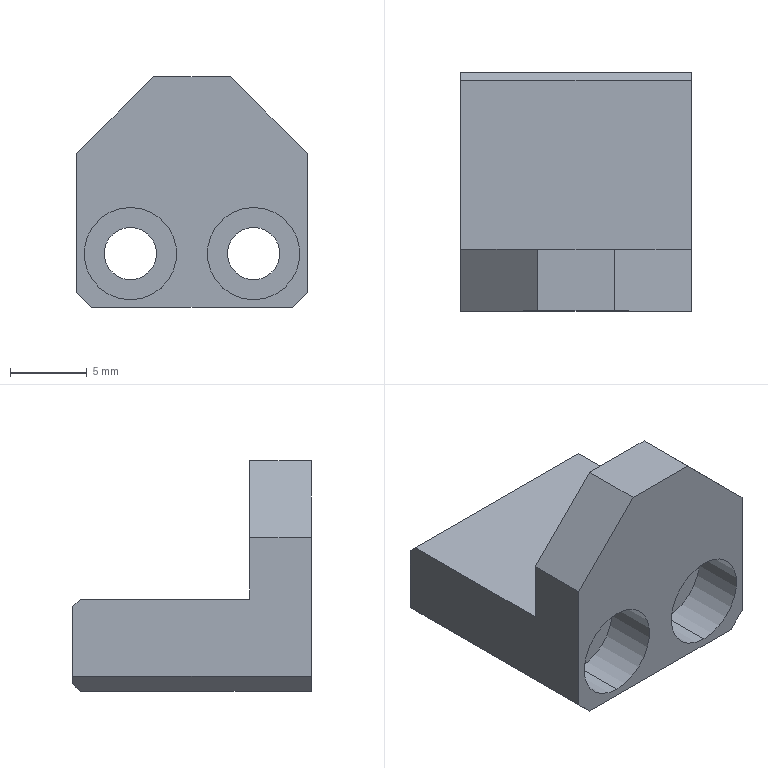Part | SolidWorks | features Chamfer 3, ICE 3, Extrusion 1, HoleWzd 1 | 1 solid | 27 faces | box 15 x 15.5 x 15 mm | volume 1371 mm3 | plane 17 | cylinder 10 | commonest cylinder face diameters 3.4 x4 6 x4 6.5 x2
STEP:
#1=CARTESIAN_POINT('',(-4.,-4.35,6.5));
#2=VERTEX_POINT('',#1);
#3=CARTESIAN_POINT('',(-4.,-4.35,0.5));
#4=VERTEX_POINT('',#3);
#5=CARTESIAN_POINT('',(-4.,-4.35,3.5));
#6=DIRECTION('',(0.,-1.,0.));
#7=DIRECTION('',(0.,0.,-1.));
#8=AXIS2_PLACEMENT_3D('',#5,#6,#7);
#9=CIRCLE('',#8,3.);
#10=EDGE_CURVE('',#2,#4,#9,.T.);
#11=ORIENTED_EDGE('',*,*,#10,.F.);
#12=CARTESIAN_POINT('',(-4.,-7.75,6.5));
#13=VERTEX_POINT('',#12);
#14=CARTESIAN_POINT('',(-4.,-7.75,6.5));
#15=DIRECTION('',(0.,-1.,0.));
#16=VECTOR('',#15,1000.);
#17=LINE('',#14,#16);
#18=EDGE_CURVE('',#2,#13,#17,.T.);
#19=ORIENTED_EDGE('',*,*,#18,.T.);
#20=CARTESIAN_POINT('',(-4.,-7.75,0.5));
#21=VERTEX_POINT('',#20);
#22=CARTESIAN_POINT('',(-4.,-7.75,3.5));
#23=DIRECTION('',(0.,-1.,0.));
#24=DIRECTION('',(0.,0.,-1.));
#25=AXIS2_PLACEMENT_3D('',#22,#23,#24);
#26=CIRCLE('',#25,3.);
#27=EDGE_CURVE('',#13,#21,#26,.T.);
#28=ORIENTED_EDGE('',*,*,#27,.T.);
#29=CARTESIAN_POINT('',(-4.,-7.75,0.5));
#30=DIRECTION('',(0.,-1.,0.));
#31=VECTOR('',#30,1000.);
#32=LINE('',#29,#31);
#33=EDGE_CURVE('',#4,#21,#32,.T.);
#34=ORIENTED_EDGE('',*,*,#33,.F.);
#35=EDGE_LOOP('',(#11,#19,#28,#34));
#36=FACE_OUTER_BOUND('',#35,.T.);
#37=CARTESIAN_POINT('',(-4.,-7.75,3.5));
#38=DIRECTION('',(0.,-1.,0.));
#39=DIRECTION('',(0.,0.,-1.));
#40=AXIS2_PLACEMENT_3D('',#37,#38,#39);
#41=CYLINDRICAL_SURFACE('',#40,3.);
#42=ADVANCED_FACE('',(#36),#41,.F.);
#43=CARTESIAN_POINT('',(-4.,7.75,5.2));
#44=VERTEX_POINT('',#43);
#45=CARTESIAN_POINT('',(-4.,7.75,1.8));
#46=VERTEX_POINT('',#45);
#47=CARTESIAN_POINT('',(-4.,7.75,3.5));
#48=DIRECTION('',(0.,-1.,0.));
#49=DIRECTION('',(0.,0.,-1.));
#50=AXIS2_PLACEMENT_3D('',#47,#48,#49);
#51=CIRCLE('',#50,1.7);
#52=EDGE_CURVE('',#44,#46,#51,.T.);
#53=ORIENTED_EDGE('',*,*,#52,.F.);
#54=CARTESIAN_POINT('',(-4.,-4.35,5.2));
#55=VERTEX_POINT('',#54);
#56=CARTESIAN_POINT('',(-4.,-7.75,5.2));
#57=DIRECTION('',(0.,-1.,0.));
#58=VECTOR('',#57,1000.);
#59=LINE('',#56,#58);
#60=EDGE_CURVE('',#44,#55,#59,.T.);
#61=ORIENTED_EDGE('',*,*,#60,.T.);
#62=CARTESIAN_POINT('',(-4.,-4.35,1.8));
#63=VERTEX_POINT('',#62);
#64=CARTESIAN_POINT('',(-4.,-4.35,3.5));
#65=DIRECTION('',(0.,-1.,0.));
#66=DIRECTION('',(0.,0.,-1.));
#67=AXIS2_PLACEMENT_3D('',#64,#65,#66);
#68=CIRCLE('',#67,1.7);
#69=EDGE_CURVE('',#55,#63,#68,.T.);
#70=ORIENTED_EDGE('',*,*,#69,.T.);
#71=CARTESIAN_POINT('',(-4.,-7.75,1.8));
#72=DIRECTION('',(0.,-1.,0.));
#73=VECTOR('',#72,1000.);
#74=LINE('',#71,#73);
#75=EDGE_CURVE('',#46,#63,#74,.T.);
#76=ORIENTED_EDGE('',*,*,#75,.F.);
#77=EDGE_LOOP('',(#53,#61,#70,#76));
#78=FACE_OUTER_BOUND('',#77,.T.);
#79=CARTESIAN_POINT('',(-4.,-7.75,3.5));
#80=DIRECTION('',(0.,-1.,0.));
#81=DIRECTION('',(0.,0.,-1.));
#82=AXIS2_PLACEMENT_3D('',#79,#80,#81);
#83=CYLINDRICAL_SURFACE('',#82,1.7);
#84=ADVANCED_FACE('',(#78),#83,.F.);
#85=CARTESIAN_POINT('',(4.,-4.35,6.5));
#86=VERTEX_POINT('',#85);
#87=CARTESIAN_POINT('',(4.,-4.35,0.5));
#88=VERTEX_POINT('',#87);
#89=CARTESIAN_POINT('',(4.,-4.35,3.5));
#90=DIRECTION('',(0.,-1.,0.));
#91=DIRECTION('',(0.,0.,-1.));
#92=AXIS2_PLACEMENT_3D('',#89,#90,#91);
#93=CIRCLE('',#92,3.);
#94=EDGE_CURVE('',#86,#88,#93,.T.);
#95=ORIENTED_EDGE('',*,*,#94,.F.);
#96=CARTESIAN_POINT('',(4.,-7.75,6.5));
#97=VERTEX_POINT('',#96);
#98=CARTESIAN_POINT('',(4.,-7.75,6.5));
#99=DIRECTION('',(0.,-1.,0.));
#100=VECTOR('',#99,1000.);
#101=LINE('',#98,#100);
#102=EDGE_CURVE('',#86,#97,#101,.T.);
#103=ORIENTED_EDGE('',*,*,#102,.T.);
#104=CARTESIAN_POINT('',(4.,-7.75,0.5));
#105=VERTEX_POINT('',#104);
#106=CARTESIAN_POINT('',(4.,-7.75,3.5));
#107=DIRECTION('',(0.,-1.,0.));
#108=DIRECTION('',(0.,0.,-1.));
#109=AXIS2_PLACEMENT_3D('',#106,#107,#108);
#110=CIRCLE('',#109,3.);
#111=EDGE_CURVE('',#97,#105,#110,.T.);
#112=ORIENTED_EDGE('',*,*,#111,.T.);
#113=CARTESIAN_POINT('',(4.,-7.75,0.5));
#114=DIRECTION('',(0.,-1.,0.));
#115=VECTOR('',#114,1000.);
#116=LINE('',#113,#115);
#117=EDGE_CURVE('',#88,#105,#116,.T.);
#118=ORIENTED_EDGE('',*,*,#117,.F.);
#119=EDGE_LOOP('',(#95,#103,#112,#118));
#120=FACE_OUTER_BOUND('',#119,.T.);
#121=CARTESIAN_POINT('',(4.,-7.75,3.5));
#122=DIRECTION('',(0.,-1.,0.));
#123=DIRECTION('',(0.,0.,-1.));
#124=AXIS2_PLACEMENT_3D('',#121,#122,#123);
#125=CYLINDRICAL_SURFACE('',#124,3.);
#126=ADVANCED_FACE('',(#120),#125,.F.);
#127=CARTESIAN_POINT('',(4.,7.75,5.2));
#128=VERTEX_POINT('',#127);
#129=CARTESIAN_POINT('',(4.,7.75,1.8));
#130=VERTEX_POINT('',#129);
#131=CARTESIAN_POINT('',(4.,7.75,3.5));
#132=DIRECTION('',(0.,-1.,0.));
#133=DIRECTION('',(0.,0.,-1.));
#134=AXIS2_PLACEMENT_3D('',#131,#132,#133);
#135=CIRCLE('',#134,1.7);
#136=EDGE_CURVE('',#128,#130,#135,.T.);
#137=ORIENTED_EDGE('',*,*,#136,.F.);
#138=CARTESIAN_POINT('',(4.,-4.35,5.2));
#139=VERTEX_POINT('',#138);
#140=CARTESIAN_POINT('',(4.,-7.75,5.2));
#141=DIRECTION('',(0.,-1.,0.));
#142=VECTOR('',#141,1000.);
#143=LINE('',#140,#142);
#144=EDGE_CURVE('',#128,#139,#143,.T.);
#145=ORIENTED_EDGE('',*,*,#144,.T.);
#146=CARTESIAN_POINT('',(4.,-4.35,1.8));
#147=VERTEX_POINT('',#146);
#148=CARTESIAN_POINT('',(4.,-4.35,3.5));
#149=DIRECTION('',(0.,-1.,0.));
#150=DIRECTION('',(0.,0.,-1.));
#151=AXIS2_PLACEMENT_3D('',#148,#149,#150);
#152=CIRCLE('',#151,1.7);
#153=EDGE_CURVE('',#139,#147,#152,.T.);
#154=ORIENTED_EDGE('',*,*,#153,.T.);
#155=CARTESIAN_POINT('',(4.,-7.75,1.8));
#156=DIRECTION('',(0.,-1.,0.));
#157=VECTOR('',#156,1000.);
#158=LINE('',#155,#157);
#159=EDGE_CURVE('',#130,#147,#158,.T.);
#160=ORIENTED_EDGE('',*,*,#159,.F.);
#161=EDGE_LOOP('',(#137,#145,#154,#160));
#162=FACE_OUTER_BOUND('',#161,.T.);
#163=CARTESIAN_POINT('',(4.,-7.75,3.5));
#164=DIRECTION('',(0.,-1.,0.));
#165=DIRECTION('',(0.,0.,-1.));
#166=AXIS2_PLACEMENT_3D('',#163,#164,#165);
#167=CYLINDRICAL_SURFACE('',#166,1.7);
#168=ADVANCED_FACE('',(#162),#167,.F.);
#169=CARTESIAN_POINT('',(0.,-4.75,7.75));
#170=VERTEX_POINT('',#169);
#171=CARTESIAN_POINT('',(0.,-4.75,14.25));
#172=VERTEX_POINT('',#171);
#173=CARTESIAN_POINT('',(0.,-4.75,11.));
#174=DIRECTION('',(0.,1.,0.));
#175=DIRECTION('',(0.,0.,1.));
#176=AXIS2_PLACEMENT_3D('',#173,#174,#175);
#177=CIRCLE('',#176,3.25);
#178=EDGE_CURVE('',#170,#172,#177,.T.);
#179=ORIENTED_EDGE('',*,*,#178,.F.);
#180=CARTESIAN_POINT('',(0.,-3.75,7.75));
#181=VERTEX_POINT('',#180);
#182=CARTESIAN_POINT('',(0.,-4.75,7.75));
#183=DIRECTION('',(0.,1.,0.));
#184=VECTOR('',#183,1000.);
#185=LINE('',#182,#184);
#186=EDGE_CURVE('',#170,#181,#185,.T.);
#187=ORIENTED_EDGE('',*,*,#186,.T.);
#188=CARTESIAN_POINT('',(0.,-3.75,14.25));
#189=VERTEX_POINT('',#188);
#190=CARTESIAN_POINT('',(0.,-3.75,11.));
#191=DIRECTION('',(0.,1.,0.));
#192=DIRECTION('',(0.,0.,1.));
#193=AXIS2_PLACEMENT_3D('',#190,#191,#192);
#194=CIRCLE('',#193,3.25);
#195=EDGE_CURVE('',#181,#189,#194,.T.);
#196=ORIENTED_EDGE('',*,*,#195,.T.);
#197=CARTESIAN_POINT('',(0.,-4.75,14.25));
#198=DIRECTION('',(0.,1.,0.));
#199=VECTOR('',#198,1000.);
#200=LINE('',#197,#199);
#201=EDGE_CURVE('',#172,#189,#200,.T.);
#202=ORIENTED_EDGE('',*,*,#201,.F.);
#203=EDGE_LOOP('',(#179,#187,#196,#202));
#204=FACE_OUTER_BOUND('',#203,.T.);
#205=CARTESIAN_POINT('',(0.,-4.75,11.));
#206=DIRECTION('',(0.,1.,0.));
#207=DIRECTION('',(0.,0.,1.));
#208=AXIS2_PLACEMENT_3D('',#205,#206,#207);
#209=CYLINDRICAL_SURFACE('',#208,3.25);
#210=ADVANCED_FACE('',(#204),#209,.F.);
#211=CARTESIAN_POINT('',(7.5,-3.75,6.));
#212=VERTEX_POINT('',#211);
#213=CARTESIAN_POINT('',(7.5,7.25,6.));
#214=VERTEX_POINT('',#213);
#215=CARTESIAN_POINT('',(7.5,-7.75,6.));
#216=DIRECTION('',(0.,1.,0.));
#217=VECTOR('',#216,1000.);
#218=LINE('',#215,#217);
#219=EDGE_CURVE('',#212,#214,#218,.T.);
#220=ORIENTED_EDGE('',*,*,#219,.T.);
#221=CARTESIAN_POINT('',(-7.5,7.25,6.));
#222=VERTEX_POINT('',#221);
#223=CARTESIAN_POINT('',(0.,7.25,6.));
#224=DIRECTION('',(-1.,0.,0.));
#225=VECTOR('',#224,1000.);
#226=LINE('',#223,#225);
#227=EDGE_CURVE('',#214,#222,#226,.T.);
#228=ORIENTED_EDGE('',*,*,#227,.T.);
#229=CARTESIAN_POINT('',(-7.5,-3.75,6.));
#230=VERTEX_POINT('',#229);
#231=CARTESIAN_POINT('',(-7.5,-7.75,6.));
#232=DIRECTION('',(0.,-1.,0.));
#233=VECTOR('',#232,1000.);
#234=LINE('',#231,#233);
#235=EDGE_CURVE('',#222,#230,#234,.T.);
#236=ORIENTED_EDGE('',*,*,#235,.T.);
#237=CARTESIAN_POINT('',(-7.5,-3.75,6.));
#238=DIRECTION('',(-1.,0.,0.));
#239=VECTOR('',#238,1000.);
#240=LINE('',#237,#239);
#241=EDGE_CURVE('',#212,#230,#240,.T.);
#242=ORIENTED_EDGE('',*,*,#241,.F.);
#243=EDGE_LOOP('',(#220,#228,#236,#242));
#244=FACE_OUTER_BOUND('',#243,.T.);
#245=CARTESIAN_POINT('',(0.,0.,6.));
#246=DIRECTION('',(0.,0.,-1.));
#247=DIRECTION('',(-1.,0.,0.));
#248=AXIS2_PLACEMENT_3D('',#245,#246,#247);
#249=PLANE('',#248);
#250=ADVANCED_FACE('',(#244),#249,.F.);
#251=CARTESIAN_POINT('',(7.5,7.75,5.5));
#252=VERTEX_POINT('',#251);
#253=CARTESIAN_POINT('',(7.5,7.75,1.));
#254=VERTEX_POINT('',#253);
#255=CARTESIAN_POINT('',(7.5,7.75,6.));
#256=DIRECTION('',(0.,0.,-1.));
#257=VECTOR('',#256,1000.);
#258=LINE('',#255,#257);
#259=EDGE_CURVE('',#252,#254,#258,.T.);
#260=ORIENTED_EDGE('',*,*,#259,.F.);
#261=CARTESIAN_POINT('',(7.5,7.25,6.));
#262=DIRECTION('',(0.,-0.7071,0.7071));
#263=VECTOR('',#262,1000.);
#264=LINE('',#261,#263);
#265=EDGE_CURVE('',#252,#214,#264,.T.);
#266=ORIENTED_EDGE('',*,*,#265,.T.);
#267=ORIENTED_EDGE('',*,*,#219,.F.);
#268=CARTESIAN_POINT('',(7.5,-3.75,10.));
#269=VERTEX_POINT('',#268);
#270=CARTESIAN_POINT('',(7.5,-3.75,15.));
#271=DIRECTION('',(0.,0.,-1.));
#272=VECTOR('',#271,1000.);
#273=LINE('',#270,#272);
#274=EDGE_CURVE('',#269,#212,#273,.T.);
#275=ORIENTED_EDGE('',*,*,#274,.F.);
#276=CARTESIAN_POINT('',(7.5,-7.75,10.));
#277=VERTEX_POINT('',#276);
#278=CARTESIAN_POINT('',(7.5,-7.75,10.));
#279=DIRECTION('',(0.,-1.,0.));
#280=VECTOR('',#279,1000.);
#281=LINE('',#278,#280);
#282=EDGE_CURVE('',#269,#277,#281,.T.);
#283=ORIENTED_EDGE('',*,*,#282,.T.);
#284=CARTESIAN_POINT('',(7.5,-7.75,1.));
#285=VERTEX_POINT('',#284);
#286=CARTESIAN_POINT('',(7.5,-7.75,6.));
#287=DIRECTION('',(0.,0.,-1.));
#288=VECTOR('',#287,1000.);
#289=LINE('',#286,#288);
#290=EDGE_CURVE('',#277,#285,#289,.T.);
#291=ORIENTED_EDGE('',*,*,#290,.T.);
#292=CARTESIAN_POINT('',(7.5,7.75,1.));
#293=DIRECTION('',(0.,1.,0.));
#294=VECTOR('',#293,1000.);
#295=LINE('',#292,#294);
#296=EDGE_CURVE('',#285,#254,#295,.T.);
#297=ORIENTED_EDGE('',*,*,#296,.T.);
#298=EDGE_LOOP('',(#260,#266,#267,#275,#283,#291,#297));
#299=FACE_OUTER_BOUND('',#298,.T.);
#300=CARTESIAN_POINT('',(7.5,-7.75,6.));
#301=DIRECTION('',(-1.,0.,0.));
#302=DIRECTION('',(0.,0.,1.));
#303=AXIS2_PLACEMENT_3D('',#300,#301,#302);
#304=PLANE('',#303);
#305=ADVANCED_FACE('',(#299),#304,.F.);
#306=CARTESIAN_POINT('',(-4.,7.75,3.5));
#307=DIRECTION('',(0.,-1.,0.));
#308=DIRECTION('',(0.,0.,-1.));
#309=AXIS2_PLACEMENT_3D('',#306,#307,#308);
#310=CIRCLE('',#309,1.7);
#311=EDGE_CURVE('',#46,#44,#310,.T.);
#312=ORIENTED_EDGE('',*,*,#311,.T.);
#313=ORIENTED_EDGE('',*,*,#52,.T.);
#314=EDGE_LOOP('',(#312,#313));
#315=FACE_BOUND('',#314,.T.);
#316=CARTESIAN_POINT('',(4.,7.75,3.5));
#317=DIRECTION('',(0.,-1.,0.));
#318=DIRECTION('',(0.,0.,-1.));
#319=AXIS2_PLACEMENT_3D('',#316,#317,#318);
#320=CIRCLE('',#319,1.7);
#321=EDGE_CURVE('',#130,#128,#320,.T.);
#322=ORIENTED_EDGE('',*,*,#321,.T.);
#323=ORIENTED_EDGE('',*,*,#136,.T.);
#324=EDGE_LOOP('',(#322,#323));
#325=FACE_BOUND('',#324,.T.);
#326=CARTESIAN_POINT('',(-7.5,7.75,5.5));
#327=VERTEX_POINT('',#326);
#328=CARTESIAN_POINT('',(-7.5,7.75,1.));
#329=VERTEX_POINT('',#328);
#330=CARTESIAN_POINT('',(-7.5,7.75,6.));
#331=DIRECTION('',(0.,0.,-1.));
#332=VECTOR('',#331,1000.);
#333=LINE('',#330,#332);
#334=EDGE_CURVE('',#327,#329,#333,.T.);
#335=ORIENTED_EDGE('',*,*,#334,.F.);
#336=CARTESIAN_POINT('',(-7.5,7.75,5.5));
#337=DIRECTION('',(1.,0.,0.));
#338=VECTOR('',#337,1000.);
#339=LINE('',#336,#338);
#340=EDGE_CURVE('',#327,#252,#339,.T.);
#341=ORIENTED_EDGE('',*,*,#340,.T.);
#342=ORIENTED_EDGE('',*,*,#259,.T.);
#343=CARTESIAN_POINT('',(7.,7.75,0.5));
#344=VERTEX_POINT('',#343);
#345=CARTESIAN_POINT('',(7.5,7.75,1.));
#346=DIRECTION('',(-0.7071,0.,-0.7071));
#347=VECTOR('',#346,1000.);
#348=LINE('',#345,#347);
#349=EDGE_CURVE('',#254,#344,#348,.T.);
#350=ORIENTED_EDGE('',*,*,#349,.T.);
#351=CARTESIAN_POINT('',(-7.,7.75,0.5));
#352=VERTEX_POINT('',#351);
#353=CARTESIAN_POINT('',(-6.5,7.75,0.5));
#354=DIRECTION('',(-1.,0.,0.));
#355=VECTOR('',#354,1000.);
#356=LINE('',#353,#355);
#357=EDGE_CURVE('',#344,#352,#356,.T.);
#358=ORIENTED_EDGE('',*,*,#357,.T.);
#359=CARTESIAN_POINT('',(-7.5,7.75,1.));
#360=DIRECTION('',(-0.7071,0.,0.7071));
#361=VECTOR('',#360,1000.);
#362=LINE('',#359,#361);
#363=EDGE_CURVE('',#352,#329,#362,.T.);
#364=ORIENTED_EDGE('',*,*,#363,.T.);
#365=EDGE_LOOP('',(#335,#341,#342,#350,#358,#364));
#366=FACE_OUTER_BOUND('',#365,.T.);
#367=CARTESIAN_POINT('',(-7.5,7.75,6.));
#368=DIRECTION('',(0.,-1.,0.));
#369=DIRECTION('',(0.,0.,-1.));
#370=AXIS2_PLACEMENT_3D('',#367,#368,#369);
#371=PLANE('',#370);
#372=ADVANCED_FACE('',(#315,#325,#366),#371,.F.);
#373=ORIENTED_EDGE('',*,*,#235,.F.);
#374=CARTESIAN_POINT('',(-7.5,7.25,6.));
#375=DIRECTION('',(0.,0.7071,-0.7071));
#376=VECTOR('',#375,1000.);
#377=LINE('',#374,#376);
#378=EDGE_CURVE('',#222,#327,#377,.T.);
#379=ORIENTED_EDGE('',*,*,#378,.T.);
#380=ORIENTED_EDGE('',*,*,#334,.T.);
#381=CARTESIAN_POINT('',(-7.5,-7.75,1.));
#382=VERTEX_POINT('',#381);
#383=CARTESIAN_POINT('',(-7.5,-7.75,1.));
#384=DIRECTION('',(0.,-1.,0.));
#385=VECTOR('',#384,1000.);
#386=LINE('',#383,#385);
#387=EDGE_CURVE('',#329,#382,#386,.T.);
#388=ORIENTED_EDGE('',*,*,#387,.T.);
#389=CARTESIAN_POINT('',(-7.5,-7.75,10.));
#390=VERTEX_POINT('',#389);
#391=CARTESIAN_POINT('',(-7.5,-7.75,6.));
#392=DIRECTION('',(0.,0.,-1.));
#393=VECTOR('',#392,1000.);
#394=LINE('',#391,#393);
#395=EDGE_CURVE('',#390,#382,#394,.T.);
#396=ORIENTED_EDGE('',*,*,#395,.F.);
#397=CARTESIAN_POINT('',(-7.5,-3.75,10.));
#398=VERTEX_POINT('',#397);
#399=CARTESIAN_POINT('',(-7.5,-7.75,10.));
#400=DIRECTION('',(0.,1.,0.));
#401=VECTOR('',#400,1000.);
#402=LINE('',#399,#401);
#403=EDGE_CURVE('',#390,#398,#402,.T.);
#404=ORIENTED_EDGE('',*,*,#403,.T.);
#405=CARTESIAN_POINT('',(-7.5,-3.75,15.));
#406=DIRECTION('',(0.,0.,-1.));
#407=VECTOR('',#406,1000.);
#408=LINE('',#405,#407);
#409=EDGE_CURVE('',#398,#230,#408,.T.);
#410=ORIENTED_EDGE('',*,*,#409,.T.);
#411=EDGE_LOOP('',(#373,#379,#380,#388,#396,#404,#410));
#412=FACE_OUTER_BOUND('',#411,.T.);
#413=CARTESIAN_POINT('',(-7.5,-7.75,6.));
#414=DIRECTION('',(1.,0.,0.));
#415=DIRECTION('',(0.,0.,-1.));
#416=AXIS2_PLACEMENT_3D('',#413,#414,#415);
#417=PLANE('',#416);
#418=ADVANCED_FACE('',(#412),#417,.F.);
#419=CARTESIAN_POINT('',(-4.,-7.75,3.5));
#420=DIRECTION('',(0.,-1.,0.));
#421=DIRECTION('',(0.,0.,-1.));
#422=AXIS2_PLACEMENT_3D('',#419,#420,#421);
#423=CIRCLE('',#422,3.);
#424=EDGE_CURVE('',#21,#13,#423,.T.);
#425=ORIENTED_EDGE('',*,*,#424,.F.);
#426=ORIENTED_EDGE('',*,*,#27,.F.);
#427=EDGE_LOOP('',(#425,#426));
#428=FACE_BOUND('',#427,.T.);
#429=CARTESIAN_POINT('',(4.,-7.75,3.5));
#430=DIRECTION('',(0.,-1.,0.));
#431=DIRECTION('',(0.,0.,-1.));
#432=AXIS2_PLACEMENT_3D('',#429,#430,#431);
#433=CIRCLE('',#432,3.);
#434=EDGE_CURVE('',#105,#97,#433,.T.);
#435=ORIENTED_EDGE('',*,*,#434,.F.);
#436=ORIENTED_EDGE('',*,*,#111,.F.);
#437=EDGE_LOOP('',(#435,#436));
#438=FACE_BOUND('',#437,.T.);
#439=CARTESIAN_POINT('',(-6.5,-7.75,0.));
#440=VERTEX_POINT('',#439);
#441=CARTESIAN_POINT('',(6.5,-7.75,0.));
#442=VERTEX_POINT('',#441);
#443=CARTESIAN_POINT('',(-7.5,-7.75,0.));
#444=DIRECTION('',(1.,0.,0.));
#445=VECTOR('',#444,1000.);
#446=LINE('',#443,#445);
#447=EDGE_CURVE('',#440,#442,#446,.T.);
#448=ORIENTED_EDGE('',*,*,#447,.T.);
#449=CARTESIAN_POINT('',(7.5,-7.75,1.));
#450=DIRECTION('',(0.7071,0.,0.7071));
#451=VECTOR('',#450,1000.);
#452=LINE('',#449,#451);
#453=EDGE_CURVE('',#442,#285,#452,.T.);
#454=ORIENTED_EDGE('',*,*,#453,.T.);
#455=ORIENTED_EDGE('',*,*,#290,.F.);
#456=CARTESIAN_POINT('',(2.5,-7.75,15.));
#457=VERTEX_POINT('',#456);
#458=CARTESIAN_POINT('',(2.5,-7.75,15.));
#459=DIRECTION('',(-0.7071,0.,0.7071));
#460=VECTOR('',#459,1000.);
#461=LINE('',#458,#460);
#462=EDGE_CURVE('',#277,#457,#461,.T.);
#463=ORIENTED_EDGE('',*,*,#462,.T.);
#464=CARTESIAN_POINT('',(-2.5,-7.75,15.));
#465=VERTEX_POINT('',#464);
#466=CARTESIAN_POINT('',(-7.5,-7.75,15.));
#467=DIRECTION('',(1.,0.,0.));
#468=VECTOR('',#467,1000.);
#469=LINE('',#466,#468);
#470=EDGE_CURVE('',#465,#457,#469,.T.);
#471=ORIENTED_EDGE('',*,*,#470,.F.);
#472=CARTESIAN_POINT('',(-2.5,-7.75,15.));
#473=DIRECTION('',(-0.7071,0.,-0.7071));
#474=VECTOR('',#473,1000.);
#475=LINE('',#472,#474);
#476=EDGE_CURVE('',#465,#390,#475,.T.);
#477=ORIENTED_EDGE('',*,*,#476,.T.);
#478=ORIENTED_EDGE('',*,*,#395,.T.);
#479=CARTESIAN_POINT('',(-7.5,-7.75,1.));
#480=DIRECTION('',(0.7071,0.,-0.7071));
#481=VECTOR('',#480,1000.);
#482=LINE('',#479,#481);
#483=EDGE_CURVE('',#382,#440,#482,.T.);
#484=ORIENTED_EDGE('',*,*,#483,.T.);
#485=EDGE_LOOP('',(#448,#454,#455,#463,#471,#477,#478,#484));
#486=FACE_OUTER_BOUND('',#485,.T.);
#487=CARTESIAN_POINT('',(-7.5,-7.75,6.));
#488=DIRECTION('',(0.,1.,0.));
#489=DIRECTION('',(0.,0.,1.));
#490=AXIS2_PLACEMENT_3D('',#487,#488,#489);
#491=PLANE('',#490);
#492=ADVANCED_FACE('',(#428,#438,#486),#491,.F.);
#493=CARTESIAN_POINT('',(-6.5,7.25,0.));
#494=VERTEX_POINT('',#493);
#495=CARTESIAN_POINT('',(-6.5,7.75,0.));
#496=DIRECTION('',(0.,1.,0.));
#497=VECTOR('',#496,1000.);
#498=LINE('',#495,#497);
#499=EDGE_CURVE('',#440,#494,#498,.T.);
#500=ORIENTED_EDGE('',*,*,#499,.T.);
#501=CARTESIAN_POINT('',(6.5,7.25,0.));
#502=VERTEX_POINT('',#501);
#503=CARTESIAN_POINT('',(6.5,7.25,0.));
#504=DIRECTION('',(1.,0.,0.));
#505=VECTOR('',#504,1000.);
#506=LINE('',#503,#505);
#507=EDGE_CURVE('',#494,#502,#506,.T.);
#508=ORIENTED_EDGE('',*,*,#507,.T.);
#509=CARTESIAN_POINT('',(6.5,-7.75,0.));
#510=DIRECTION('',(0.,-1.,0.));
#511=VECTOR('',#510,1000.);
#512=LINE('',#509,#511);
#513=EDGE_CURVE('',#502,#442,#512,.T.);
#514=ORIENTED_EDGE('',*,*,#513,.T.);
#515=ORIENTED_EDGE('',*,*,#447,.F.);
#516=EDGE_LOOP('',(#500,#508,#514,#515));
#517=FACE_OUTER_BOUND('',#516,.T.);
#518=CARTESIAN_POINT('',(0.,0.,0.));
#519=DIRECTION('',(0.,0.,-1.));
#520=DIRECTION('',(-1.,0.,0.));
#521=AXIS2_PLACEMENT_3D('',#518,#519,#520);
#522=PLANE('',#521);
#523=ADVANCED_FACE('',(#517),#522,.T.);
#524=CARTESIAN_POINT('',(0.,-3.75,11.));
#525=DIRECTION('',(0.,1.,0.));
#526=DIRECTION('',(0.,0.,1.));
#527=AXIS2_PLACEMENT_3D('',#524,#525,#526);
#528=CIRCLE('',#527,3.25);
#529=EDGE_CURVE('',#189,#181,#528,.T.);
#530=ORIENTED_EDGE('',*,*,#529,.F.);
#531=ORIENTED_EDGE('',*,*,#195,.F.);
#532=EDGE_LOOP('',(#530,#531));
#533=FACE_BOUND('',#532,.T.);
#534=ORIENTED_EDGE('',*,*,#409,.F.);
#535=CARTESIAN_POINT('',(-2.5,-3.75,15.));
#536=VERTEX_POINT('',#535);
#537=CARTESIAN_POINT('',(-2.5,-3.75,15.));
#538=DIRECTION('',(0.7071,0.,0.7071));
#539=VECTOR('',#538,1000.);
#540=LINE('',#537,#539);
#541=EDGE_CURVE('',#398,#536,#540,.T.);
#542=ORIENTED_EDGE('',*,*,#541,.T.);
#543=CARTESIAN_POINT('',(2.5,-3.75,15.));
#544=VERTEX_POINT('',#543);
#545=CARTESIAN_POINT('',(-7.5,-3.75,15.));
#546=DIRECTION('',(-1.,0.,0.));
#547=VECTOR('',#546,1000.);
#548=LINE('',#545,#547);
#549=EDGE_CURVE('',#544,#536,#548,.T.);
#550=ORIENTED_EDGE('',*,*,#549,.F.);
#551=CARTESIAN_POINT('',(2.5,-3.75,15.));
#552=DIRECTION('',(0.7071,0.,-0.7071));
#553=VECTOR('',#552,1000.);
#554=LINE('',#551,#553);
#555=EDGE_CURVE('',#544,#269,#554,.T.);
#556=ORIENTED_EDGE('',*,*,#555,.T.);
#557=ORIENTED_EDGE('',*,*,#274,.T.);
#558=ORIENTED_EDGE('',*,*,#241,.T.);
#559=EDGE_LOOP('',(#534,#542,#550,#556,#557,#558));
#560=FACE_OUTER_BOUND('',#559,.T.);
#561=CARTESIAN_POINT('',(-7.5,-3.75,15.));
#562=DIRECTION('',(0.,-1.,0.));
#563=DIRECTION('',(0.,0.,-1.));
#564=AXIS2_PLACEMENT_3D('',#561,#562,#563);
#565=PLANE('',#564);
#566=ADVANCED_FACE('',(#533,#560),#565,.F.);
#567=ORIENTED_EDGE('',*,*,#549,.T.);
#568=CARTESIAN_POINT('',(-2.5,0.,15.));
#569=DIRECTION('',(0.,-1.,0.));
#570=VECTOR('',#569,1000.);
#571=LINE('',#568,#570);
#572=EDGE_CURVE('',#536,#465,#571,.T.);
#573=ORIENTED_EDGE('',*,*,#572,.T.);
#574=ORIENTED_EDGE('',*,*,#470,.T.);
#575=CARTESIAN_POINT('',(2.5,0.,15.));
#576=DIRECTION('',(0.,1.,0.));
#577=VECTOR('',#576,1000.);
#578=LINE('',#575,#577);
#579=EDGE_CURVE('',#457,#544,#578,.T.);
#580=ORIENTED_EDGE('',*,*,#579,.T.);
#581=EDGE_LOOP('',(#567,#573,#574,#580));
#582=FACE_OUTER_BOUND('',#581,.T.);
#583=CARTESIAN_POINT('',(0.,0.,15.));
#584=DIRECTION('',(0.,0.,-1.));
#585=DIRECTION('',(-1.,0.,0.));
#586=AXIS2_PLACEMENT_3D('',#583,#584,#585);
#587=PLANE('',#586);
#588=ADVANCED_FACE('',(#582),#587,.F.);
#589=ORIENTED_EDGE('',*,*,#186,.F.);
#590=CARTESIAN_POINT('',(0.,-4.75,11.));
#591=DIRECTION('',(0.,1.,0.));
#592=DIRECTION('',(0.,0.,1.));
#593=AXIS2_PLACEMENT_3D('',#590,#591,#592);
#594=CIRCLE('',#593,3.25);
#595=EDGE_CURVE('',#172,#170,#594,.T.);
#596=ORIENTED_EDGE('',*,*,#595,.F.);
#597=ORIENTED_EDGE('',*,*,#201,.T.);
#598=ORIENTED_EDGE('',*,*,#529,.T.);
#599=EDGE_LOOP('',(#589,#596,#597,#598));
#600=FACE_OUTER_BOUND('',#599,.T.);
#601=CARTESIAN_POINT('',(0.,-4.75,11.));
#602=DIRECTION('',(0.,1.,0.));
#603=DIRECTION('',(0.,0.,1.));
#604=AXIS2_PLACEMENT_3D('',#601,#602,#603);
#605=CYLINDRICAL_SURFACE('',#604,3.25);
#606=ADVANCED_FACE('',(#600),#605,.F.);
#607=ORIENTED_EDGE('',*,*,#595,.T.);
#608=ORIENTED_EDGE('',*,*,#178,.T.);
#609=EDGE_LOOP('',(#607,#608));
#610=FACE_OUTER_BOUND('',#609,.T.);
#611=CARTESIAN_POINT('',(0.,-4.75,11.));
#612=DIRECTION('',(0.,1.,0.));
#613=DIRECTION('',(0.,0.,1.));
#614=AXIS2_PLACEMENT_3D('',#611,#612,#613);
#615=PLANE('',#614);
#616=ADVANCED_FACE('',(#610),#615,.T.);
#617=ORIENTED_EDGE('',*,*,#144,.F.);
#618=ORIENTED_EDGE('',*,*,#321,.F.);
#619=ORIENTED_EDGE('',*,*,#159,.T.);
#620=CARTESIAN_POINT('',(4.,-4.35,3.5));
#621=DIRECTION('',(0.,-1.,0.));
#622=DIRECTION('',(0.,0.,-1.));
#623=AXIS2_PLACEMENT_3D('',#620,#621,#622);
#624=CIRCLE('',#623,1.7);
#625=EDGE_CURVE('',#147,#139,#624,.T.);
#626=ORIENTED_EDGE('',*,*,#625,.T.);
#627=EDGE_LOOP('',(#617,#618,#619,#626));
#628=FACE_OUTER_BOUND('',#627,.T.);
#629=CARTESIAN_POINT('',(4.,-7.75,3.5));
#630=DIRECTION('',(0.,-1.,0.));
#631=DIRECTION('',(0.,0.,-1.));
#632=AXIS2_PLACEMENT_3D('',#629,#630,#631);
#633=CYLINDRICAL_SURFACE('',#632,1.7);
#634=ADVANCED_FACE('',(#628),#633,.F.);
#635=ORIENTED_EDGE('',*,*,#625,.F.);
#636=ORIENTED_EDGE('',*,*,#153,.F.);
#637=EDGE_LOOP('',(#635,#636));
#638=FACE_BOUND('',#637,.T.);
#639=CARTESIAN_POINT('',(4.,-4.35,3.5));
#640=DIRECTION('',(0.,-1.,0.));
#641=DIRECTION('',(0.,0.,-1.));
#642=AXIS2_PLACEMENT_3D('',#639,#640,#641);
#643=CIRCLE('',#642,3.);
#644=EDGE_CURVE('',#88,#86,#643,.T.);
#645=ORIENTED_EDGE('',*,*,#644,.T.);
#646=ORIENTED_EDGE('',*,*,#94,.T.);
#647=EDGE_LOOP('',(#645,#646));
#648=FACE_OUTER_BOUND('',#647,.T.);
#649=CARTESIAN_POINT('',(5.7,-4.35,3.5));
#650=DIRECTION('',(0.,1.,0.));
#651=DIRECTION('',(0.,0.,1.));
#652=AXIS2_PLACEMENT_3D('',#649,#650,#651);
#653=PLANE('',#652);
#654=ADVANCED_FACE('',(#638,#648),#653,.F.);
#655=ORIENTED_EDGE('',*,*,#102,.F.);
#656=ORIENTED_EDGE('',*,*,#644,.F.);
#657=ORIENTED_EDGE('',*,*,#117,.T.);
#658=ORIENTED_EDGE('',*,*,#434,.T.);
#659=EDGE_LOOP('',(#655,#656,#657,#658));
#660=FACE_OUTER_BOUND('',#659,.T.);
#661=CARTESIAN_POINT('',(4.,-7.75,3.5));
#662=DIRECTION('',(0.,-1.,0.));
#663=DIRECTION('',(0.,0.,-1.));
#664=AXIS2_PLACEMENT_3D('',#661,#662,#663);
#665=CYLINDRICAL_SURFACE('',#664,3.);
#666=ADVANCED_FACE('',(#660),#665,.F.);
#667=ORIENTED_EDGE('',*,*,#60,.F.);
#668=ORIENTED_EDGE('',*,*,#311,.F.);
#669=ORIENTED_EDGE('',*,*,#75,.T.);
#670=CARTESIAN_POINT('',(-4.,-4.35,3.5));
#671=DIRECTION('',(0.,-1.,0.));
#672=DIRECTION('',(0.,0.,-1.));
#673=AXIS2_PLACEMENT_3D('',#670,#671,#672);
#674=CIRCLE('',#673,1.7);
#675=EDGE_CURVE('',#63,#55,#674,.T.);
#676=ORIENTED_EDGE('',*,*,#675,.T.);
#677=EDGE_LOOP('',(#667,#668,#669,#676));
#678=FACE_OUTER_BOUND('',#677,.T.);
#679=CARTESIAN_POINT('',(-4.,-7.75,3.5));
#680=DIRECTION('',(0.,-1.,0.));
#681=DIRECTION('',(0.,0.,-1.));
#682=AXIS2_PLACEMENT_3D('',#679,#680,#681);
#683=CYLINDRICAL_SURFACE('',#682,1.7);
#684=ADVANCED_FACE('',(#678),#683,.F.);
#685=ORIENTED_EDGE('',*,*,#675,.F.);
#686=ORIENTED_EDGE('',*,*,#69,.F.);
#687=EDGE_LOOP('',(#685,#686));
#688=FACE_BOUND('',#687,.T.);
#689=CARTESIAN_POINT('',(-4.,-4.35,3.5));
#690=DIRECTION('',(0.,-1.,0.));
#691=DIRECTION('',(0.,0.,-1.));
#692=AXIS2_PLACEMENT_3D('',#689,#690,#691);
#693=CIRCLE('',#692,3.);
#694=EDGE_CURVE('',#4,#2,#693,.T.);
#695=ORIENTED_EDGE('',*,*,#694,.T.);
#696=ORIENTED_EDGE('',*,*,#10,.T.);
#697=EDGE_LOOP('',(#695,#696));
#698=FACE_OUTER_BOUND('',#697,.T.);
#699=CARTESIAN_POINT('',(-2.3,-4.35,3.5));
#700=DIRECTION('',(0.,1.,0.));
#701=DIRECTION('',(0.,0.,1.));
#702=AXIS2_PLACEMENT_3D('',#699,#700,#701);
#703=PLANE('',#702);
#704=ADVANCED_FACE('',(#688,#698),#703,.F.);
#705=ORIENTED_EDGE('',*,*,#18,.F.);
#706=ORIENTED_EDGE('',*,*,#694,.F.);
#707=ORIENTED_EDGE('',*,*,#33,.T.);
#708=ORIENTED_EDGE('',*,*,#424,.T.);
#709=EDGE_LOOP('',(#705,#706,#707,#708));
#710=FACE_OUTER_BOUND('',#709,.T.);
#711=CARTESIAN_POINT('',(-4.,-7.75,3.5));
#712=DIRECTION('',(0.,-1.,0.));
#713=DIRECTION('',(0.,0.,-1.));
#714=AXIS2_PLACEMENT_3D('',#711,#712,#713);
#715=CYLINDRICAL_SURFACE('',#714,3.);
#716=ADVANCED_FACE('',(#710),#715,.F.);
#717=ORIENTED_EDGE('',*,*,#541,.F.);
#718=ORIENTED_EDGE('',*,*,#403,.F.);
#719=ORIENTED_EDGE('',*,*,#476,.F.);
#720=ORIENTED_EDGE('',*,*,#572,.F.);
#721=EDGE_LOOP('',(#717,#718,#719,#720));
#722=FACE_OUTER_BOUND('',#721,.T.);
#723=CARTESIAN_POINT('',(-2.5,0.,15.));
#724=DIRECTION('',(0.7071,0.,-0.7071));
#725=DIRECTION('',(0.,-1.,0.));
#726=AXIS2_PLACEMENT_3D('',#723,#724,#725);
#727=PLANE('',#726);
#728=ADVANCED_FACE('',(#722),#727,.F.);
#729=ORIENTED_EDGE('',*,*,#462,.F.);
#730=ORIENTED_EDGE('',*,*,#282,.F.);
#731=ORIENTED_EDGE('',*,*,#555,.F.);
#732=ORIENTED_EDGE('',*,*,#579,.F.);
#733=EDGE_LOOP('',(#729,#730,#731,#732));
#734=FACE_OUTER_BOUND('',#733,.T.);
#735=CARTESIAN_POINT('',(2.5,0.,15.));
#736=DIRECTION('',(-0.7071,0.,-0.7071));
#737=DIRECTION('',(0.,1.,0.));
#738=AXIS2_PLACEMENT_3D('',#735,#736,#737);
#739=PLANE('',#738);
#740=ADVANCED_FACE('',(#734),#739,.F.);
#741=ORIENTED_EDGE('',*,*,#513,.F.);
#742=CARTESIAN_POINT('',(2.167,2.917,-4.333));
#743=DIRECTION('',(0.5774,0.5774,0.5774));
#744=VECTOR('',#743,1000.);
#745=LINE('',#742,#744);
#746=EDGE_CURVE('',#502,#344,#745,.T.);
#747=ORIENTED_EDGE('',*,*,#746,.T.);
#748=ORIENTED_EDGE('',*,*,#349,.F.);
#749=ORIENTED_EDGE('',*,*,#296,.F.);
#750=ORIENTED_EDGE('',*,*,#453,.F.);
#751=EDGE_LOOP('',(#741,#747,#748,#749,#750));
#752=FACE_OUTER_BOUND('',#751,.T.);
#753=CARTESIAN_POINT('',(7.5,-7.75,1.));
#754=DIRECTION('',(0.7071,0.,-0.7071));
#755=DIRECTION('',(0.,-1.,0.));
#756=AXIS2_PLACEMENT_3D('',#753,#754,#755);
#757=PLANE('',#756);
#758=ADVANCED_FACE('',(#752),#757,.T.);
#759=ORIENTED_EDGE('',*,*,#363,.F.);
#760=CARTESIAN_POINT('',(-2.167,2.917,-4.333));
#761=DIRECTION('',(0.5774,-0.5774,-0.5774));
#762=VECTOR('',#761,1000.);
#763=LINE('',#760,#762);
#764=EDGE_CURVE('',#352,#494,#763,.T.);
#765=ORIENTED_EDGE('',*,*,#764,.T.);
#766=ORIENTED_EDGE('',*,*,#499,.F.);
#767=ORIENTED_EDGE('',*,*,#483,.F.);
#768=ORIENTED_EDGE('',*,*,#387,.F.);
#769=EDGE_LOOP('',(#759,#765,#766,#767,#768));
#770=FACE_OUTER_BOUND('',#769,.T.);
#771=CARTESIAN_POINT('',(-7.5,-7.75,1.));
#772=DIRECTION('',(-0.7071,0.,-0.7071));
#773=DIRECTION('',(0.,1.,0.));
#774=AXIS2_PLACEMENT_3D('',#771,#772,#773);
#775=PLANE('',#774);
#776=ADVANCED_FACE('',(#770),#775,.T.);
#777=ORIENTED_EDGE('',*,*,#265,.F.);
#778=ORIENTED_EDGE('',*,*,#340,.F.);
#779=ORIENTED_EDGE('',*,*,#378,.F.);
#780=ORIENTED_EDGE('',*,*,#227,.F.);
#781=EDGE_LOOP('',(#777,#778,#779,#780));
#782=FACE_OUTER_BOUND('',#781,.T.);
#783=CARTESIAN_POINT('',(0.,7.25,6.));
#784=DIRECTION('',(0.,-0.7071,-0.7071));
#785=DIRECTION('',(-1.,0.,0.));
#786=AXIS2_PLACEMENT_3D('',#783,#784,#785);
#787=PLANE('',#786);
#788=ADVANCED_FACE('',(#782),#787,.F.);
#789=ORIENTED_EDGE('',*,*,#746,.F.);
#790=ORIENTED_EDGE('',*,*,#507,.F.);
#791=ORIENTED_EDGE('',*,*,#764,.F.);
#792=ORIENTED_EDGE('',*,*,#357,.F.);
#793=EDGE_LOOP('',(#789,#790,#791,#792));
#794=FACE_OUTER_BOUND('',#793,.T.);
#795=CARTESIAN_POINT('',(-7.5,7.75,0.5));
#796=DIRECTION('',(0.,0.7071,-0.7071));
#797=DIRECTION('',(1.,0.,0.));
#798=AXIS2_PLACEMENT_3D('',#795,#796,#797);
#799=PLANE('',#798);
#800=ADVANCED_FACE('',(#794),#799,.T.);
#801=CLOSED_SHELL('',(#42,#84,#126,#168,#210,#250,#305,#372,#418,#492,#523,#566,#588,#606,#616,#634,#654,#666,#684,#704,#716,#728,#740,#758,#776,#788,#800));
#802=MANIFOLD_SOLID_BREP('',#801);
#803=CARTESIAN_POINT('',(0.,0.,0.));
#804=DIRECTION('',(0.,0.,1.));
#805=DIRECTION('',(1.,0.,0.));
#806=AXIS2_PLACEMENT_3D('',#803,#804,#805);
#807=(LENGTH_UNIT()NAMED_UNIT(*)SI_UNIT(.MILLI.,.METRE.));
#808=UNCERTAINTY_MEASURE_WITH_UNIT(LENGTH_MEASURE(0.00001),#807,'','');
#809=(NAMED_UNIT(*)PLANE_ANGLE_UNIT()SI_UNIT($,.RADIAN.));
#810=(NAMED_UNIT(*)SI_UNIT($,.STERADIAN.)SOLID_ANGLE_UNIT());
#811=(GEOMETRIC_REPRESENTATION_CONTEXT(3)GLOBAL_UNCERTAINTY_ASSIGNED_CONTEXT((#808))GLOBAL_UNIT_ASSIGNED_CONTEXT((#807,#809,#810))REPRESENTATION_CONTEXT('',''));
#812=ADVANCED_BREP_SHAPE_REPRESENTATION('',(#802,#806),#811);